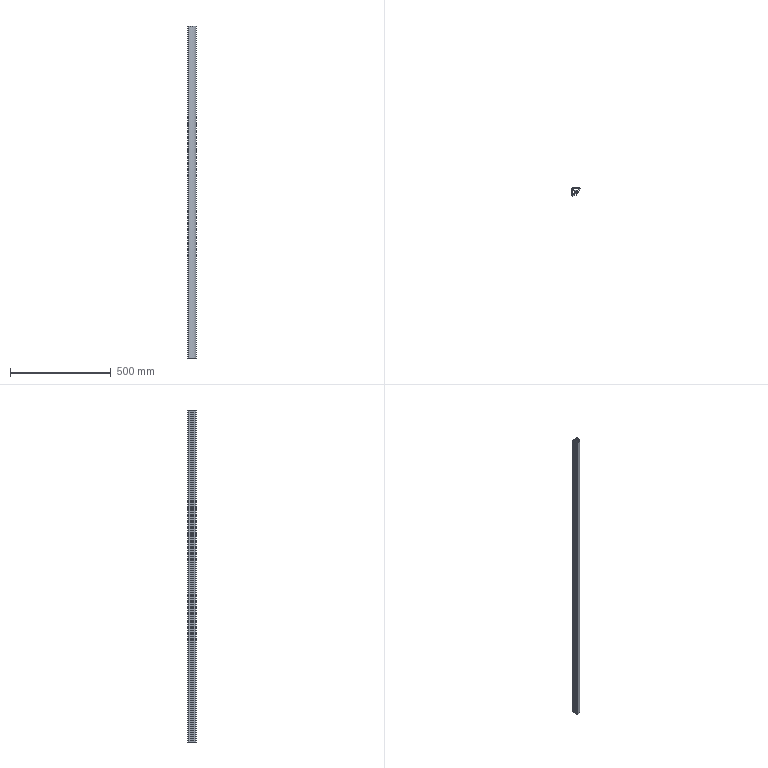Part | 1 solid | 59 faces | box 39.857 x 39.857 x 1650 mm | volume 804681 mm3 | plane 48 | cylinder 11 | commonest cylinder face diameters 5 x3 9 x3 6.8 x2 66.41 x1 76.531 x1 80 x1